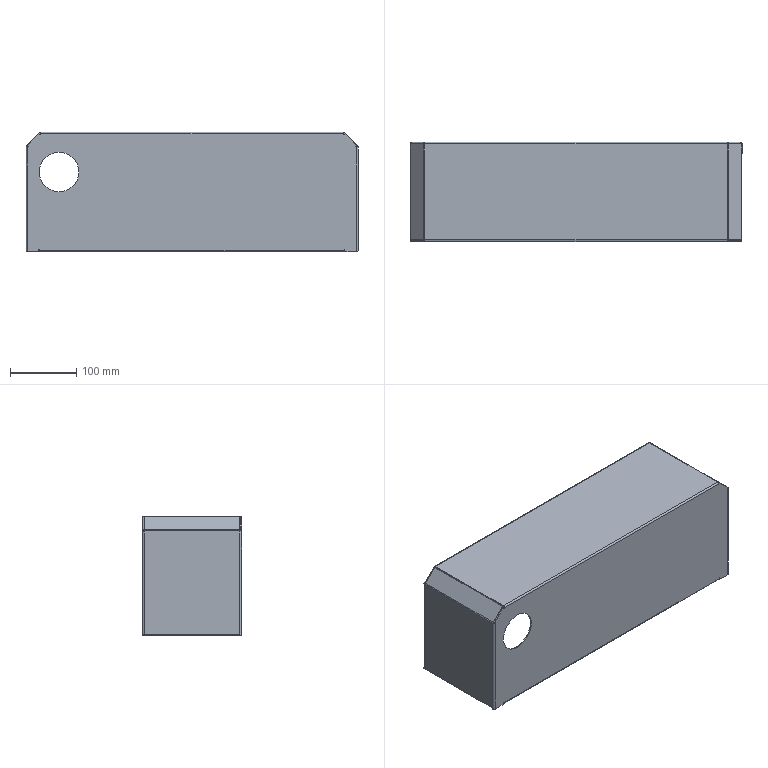Part | STEP file | Control Box Upper 1 | 1 solid | 134 faces | box 502 x 150 x 180.5 mm | volume 475305 mm3 | plane 92 | cylinder 34 | spline 8 | commonest cylinder face diameters 1 x12 5 x12 7 x6 60 x2 0.2 x1 4.2 x1